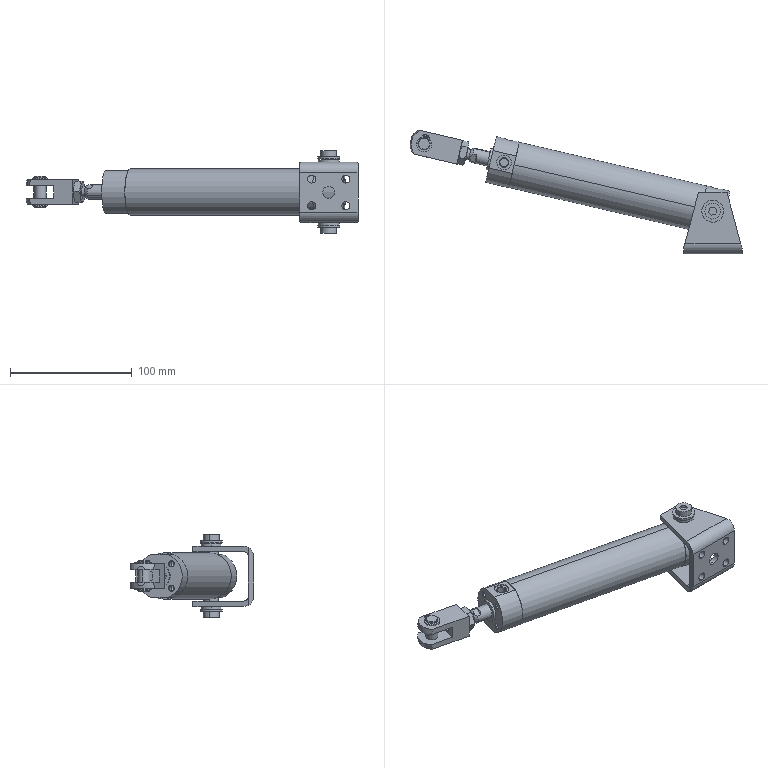Part | SolidWorks | features AEMSimFeature 1, CompositeCurve 1 | 5 solids | 303 faces | box 272.662 x 101.563 x 67.7 mm | volume 211806 mm3 | cylinder 132 | plane 107 | cone 62 | torus 2 | commonest cylinder face diameters 4.134 x16 12 x16 10 x14 1.2 x8 2 x8 6.6 x8